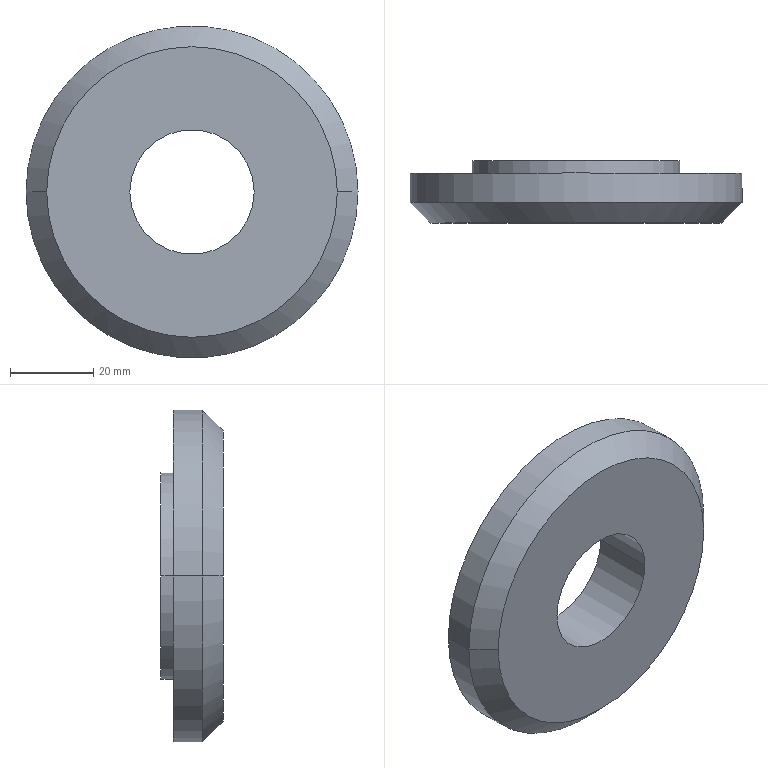Part | SolidWorks | features Revolution 1 | 1 solid | 14 faces | box 80 x 15 x 80 mm | volume 46941 mm3 | cylinder 8 | plane 4 | cone 2 | commonest cylinder face diameters 30 x2 50 x2 70 x2 80 x2
STEP:
#1=CARTESIAN_POINT('',(25.,532.,0.));
#2=VERTEX_POINT('',#1);
#3=CARTESIAN_POINT('',(-25.,532.,0.));
#4=VERTEX_POINT('',#3);
#5=CARTESIAN_POINT('',(0.,532.,0.));
#6=DIRECTION('',(0.,-1.,0.));
#7=DIRECTION('',(1.,0.,0.));
#8=AXIS2_PLACEMENT_3D('',#5,#6,#7);
#9=CIRCLE('',#8,25.);
#10=EDGE_CURVE('',#2,#4,#9,.T.);
#11=ORIENTED_EDGE('',*,*,#10,.T.);
#12=CARTESIAN_POINT('',(-25.,526.,0.));
#13=VERTEX_POINT('',#12);
#14=CARTESIAN_POINT('',(-25.,517.,0.));
#15=DIRECTION('',(0.,-1.,0.));
#16=VECTOR('',#15,1000.);
#17=LINE('',#14,#16);
#18=EDGE_CURVE('',#4,#13,#17,.T.);
#19=ORIENTED_EDGE('',*,*,#18,.T.);
#20=CARTESIAN_POINT('',(25.,526.,0.));
#21=VERTEX_POINT('',#20);
#22=CARTESIAN_POINT('',(0.,526.,0.));
#23=DIRECTION('',(0.,-1.,0.));
#24=DIRECTION('',(1.,0.,0.));
#25=AXIS2_PLACEMENT_3D('',#22,#23,#24);
#26=CIRCLE('',#25,25.);
#27=EDGE_CURVE('',#21,#13,#26,.T.);
#28=ORIENTED_EDGE('',*,*,#27,.F.);
#29=CARTESIAN_POINT('',(25.,517.,0.));
#30=DIRECTION('',(0.,-1.,0.));
#31=VECTOR('',#30,1000.);
#32=LINE('',#29,#31);
#33=EDGE_CURVE('',#2,#21,#32,.T.);
#34=ORIENTED_EDGE('',*,*,#33,.F.);
#35=EDGE_LOOP('',(#11,#19,#28,#34));
#36=FACE_OUTER_BOUND('',#35,.T.);
#37=CARTESIAN_POINT('',(0.,517.,0.));
#38=DIRECTION('',(0.,-1.,0.));
#39=DIRECTION('',(1.,0.,0.));
#40=AXIS2_PLACEMENT_3D('',#37,#38,#39);
#41=CYLINDRICAL_SURFACE('',#40,25.);
#42=ADVANCED_FACE('',(#36),#41,.T.);
#43=CARTESIAN_POINT('',(-35.,529.,0.));
#44=VERTEX_POINT('',#43);
#45=CARTESIAN_POINT('',(35.,529.,0.));
#46=VERTEX_POINT('',#45);
#47=CARTESIAN_POINT('',(0.,529.,0.));
#48=DIRECTION('',(0.,-1.,0.));
#49=DIRECTION('',(1.,0.,0.));
#50=AXIS2_PLACEMENT_3D('',#47,#48,#49);
#51=CIRCLE('',#50,35.);
#52=EDGE_CURVE('',#44,#46,#51,.T.);
#53=ORIENTED_EDGE('',*,*,#52,.F.);
#54=CARTESIAN_POINT('',(-35.,526.,0.));
#55=VERTEX_POINT('',#54);
#56=CARTESIAN_POINT('',(-35.,517.,0.));
#57=DIRECTION('',(0.,-1.,0.));
#58=VECTOR('',#57,1000.);
#59=LINE('',#56,#58);
#60=EDGE_CURVE('',#44,#55,#59,.T.);
#61=ORIENTED_EDGE('',*,*,#60,.T.);
#62=CARTESIAN_POINT('',(35.,526.,0.));
#63=VERTEX_POINT('',#62);
#64=CARTESIAN_POINT('',(0.,526.,0.));
#65=DIRECTION('',(0.,-1.,0.));
#66=DIRECTION('',(1.,0.,0.));
#67=AXIS2_PLACEMENT_3D('',#64,#65,#66);
#68=CIRCLE('',#67,35.);
#69=EDGE_CURVE('',#55,#63,#68,.T.);
#70=ORIENTED_EDGE('',*,*,#69,.T.);
#71=CARTESIAN_POINT('',(35.,517.,0.));
#72=DIRECTION('',(0.,-1.,0.));
#73=VECTOR('',#72,1000.);
#74=LINE('',#71,#73);
#75=EDGE_CURVE('',#46,#63,#74,.T.);
#76=ORIENTED_EDGE('',*,*,#75,.F.);
#77=EDGE_LOOP('',(#53,#61,#70,#76));
#78=FACE_OUTER_BOUND('',#77,.T.);
#79=CARTESIAN_POINT('',(0.,517.,0.));
#80=DIRECTION('',(0.,-1.,0.));
#81=DIRECTION('',(1.,0.,0.));
#82=AXIS2_PLACEMENT_3D('',#79,#80,#81);
#83=CYLINDRICAL_SURFACE('',#82,35.);
#84=ADVANCED_FACE('',(#78),#83,.F.);
#85=CARTESIAN_POINT('',(40.,529.,0.));
#86=VERTEX_POINT('',#85);
#87=CARTESIAN_POINT('',(-40.,529.,0.));
#88=VERTEX_POINT('',#87);
#89=CARTESIAN_POINT('',(0.,529.,0.));
#90=DIRECTION('',(0.,-1.,0.));
#91=DIRECTION('',(1.,0.,0.));
#92=AXIS2_PLACEMENT_3D('',#89,#90,#91);
#93=CIRCLE('',#92,40.);
#94=EDGE_CURVE('',#86,#88,#93,.T.);
#95=ORIENTED_EDGE('',*,*,#94,.T.);
#96=CARTESIAN_POINT('',(-40.,522.,0.));
#97=VERTEX_POINT('',#96);
#98=CARTESIAN_POINT('',(-40.,517.,0.));
#99=DIRECTION('',(0.,-1.,0.));
#100=VECTOR('',#99,1000.);
#101=LINE('',#98,#100);
#102=EDGE_CURVE('',#88,#97,#101,.T.);
#103=ORIENTED_EDGE('',*,*,#102,.T.);
#104=CARTESIAN_POINT('',(40.,522.,0.));
#105=VERTEX_POINT('',#104);
#106=CARTESIAN_POINT('',(0.,522.,0.));
#107=DIRECTION('',(0.,-1.,0.));
#108=DIRECTION('',(1.,0.,0.));
#109=AXIS2_PLACEMENT_3D('',#106,#107,#108);
#110=CIRCLE('',#109,40.);
#111=EDGE_CURVE('',#105,#97,#110,.T.);
#112=ORIENTED_EDGE('',*,*,#111,.F.);
#113=CARTESIAN_POINT('',(40.,517.,0.));
#114=DIRECTION('',(0.,-1.,0.));
#115=VECTOR('',#114,1000.);
#116=LINE('',#113,#115);
#117=EDGE_CURVE('',#86,#105,#116,.T.);
#118=ORIENTED_EDGE('',*,*,#117,.F.);
#119=EDGE_LOOP('',(#95,#103,#112,#118));
#120=FACE_OUTER_BOUND('',#119,.T.);
#121=CARTESIAN_POINT('',(0.,517.,0.));
#122=DIRECTION('',(0.,-1.,0.));
#123=DIRECTION('',(1.,0.,0.));
#124=AXIS2_PLACEMENT_3D('',#121,#122,#123);
#125=CYLINDRICAL_SURFACE('',#124,40.);
#126=ADVANCED_FACE('',(#120),#125,.T.);
#127=CARTESIAN_POINT('',(35.,517.,0.));
#128=VERTEX_POINT('',#127);
#129=CARTESIAN_POINT('',(-35.,517.,0.));
#130=VERTEX_POINT('',#129);
#131=CARTESIAN_POINT('',(0.,517.,0.));
#132=DIRECTION('',(0.,-1.,0.));
#133=DIRECTION('',(1.,0.,0.));
#134=AXIS2_PLACEMENT_3D('',#131,#132,#133);
#135=CIRCLE('',#134,35.);
#136=EDGE_CURVE('',#128,#130,#135,.T.);
#137=ORIENTED_EDGE('',*,*,#136,.F.);
#138=CARTESIAN_POINT('',(35.,517.,0.));
#139=DIRECTION('',(0.7071,0.7071,0.));
#140=VECTOR('',#139,1000.);
#141=LINE('',#138,#140);
#142=EDGE_CURVE('',#128,#105,#141,.T.);
#143=ORIENTED_EDGE('',*,*,#142,.T.);
#144=ORIENTED_EDGE('',*,*,#111,.T.);
#145=CARTESIAN_POINT('',(-35.,517.,0.));
#146=DIRECTION('',(-0.7071,0.7071,0.));
#147=VECTOR('',#146,1000.);
#148=LINE('',#145,#147);
#149=EDGE_CURVE('',#130,#97,#148,.T.);
#150=ORIENTED_EDGE('',*,*,#149,.F.);
#151=EDGE_LOOP('',(#137,#143,#144,#150));
#152=FACE_OUTER_BOUND('',#151,.T.);
#153=CARTESIAN_POINT('',(0.,517.,0.));
#154=DIRECTION('',(0.,1.,0.));
#155=DIRECTION('',(-1.,0.,0.));
#156=AXIS2_PLACEMENT_3D('',#153,#154,#155);
#157=CONICAL_SURFACE('',#156,35.,0.7854);
#158=ADVANCED_FACE('',(#152),#157,.T.);
#159=CARTESIAN_POINT('',(-15.,532.,0.));
#160=VERTEX_POINT('',#159);
#161=CARTESIAN_POINT('',(15.,532.,0.));
#162=VERTEX_POINT('',#161);
#163=CARTESIAN_POINT('',(0.,532.,0.));
#164=DIRECTION('',(0.,-1.,0.));
#165=DIRECTION('',(1.,0.,0.));
#166=AXIS2_PLACEMENT_3D('',#163,#164,#165);
#167=CIRCLE('',#166,15.);
#168=EDGE_CURVE('',#160,#162,#167,.T.);
#169=ORIENTED_EDGE('',*,*,#168,.F.);
#170=CARTESIAN_POINT('',(-15.,517.,0.));
#171=VERTEX_POINT('',#170);
#172=CARTESIAN_POINT('',(-15.,517.,0.));
#173=DIRECTION('',(0.,-1.,0.));
#174=VECTOR('',#173,1000.);
#175=LINE('',#172,#174);
#176=EDGE_CURVE('',#160,#171,#175,.T.);
#177=ORIENTED_EDGE('',*,*,#176,.T.);
#178=CARTESIAN_POINT('',(15.,517.,0.));
#179=VERTEX_POINT('',#178);
#180=CARTESIAN_POINT('',(0.,517.,0.));
#181=DIRECTION('',(0.,-1.,0.));
#182=DIRECTION('',(1.,0.,0.));
#183=AXIS2_PLACEMENT_3D('',#180,#181,#182);
#184=CIRCLE('',#183,15.);
#185=EDGE_CURVE('',#171,#179,#184,.T.);
#186=ORIENTED_EDGE('',*,*,#185,.T.);
#187=CARTESIAN_POINT('',(15.,517.,0.));
#188=DIRECTION('',(0.,-1.,0.));
#189=VECTOR('',#188,1000.);
#190=LINE('',#187,#189);
#191=EDGE_CURVE('',#162,#179,#190,.T.);
#192=ORIENTED_EDGE('',*,*,#191,.F.);
#193=EDGE_LOOP('',(#169,#177,#186,#192));
#194=FACE_OUTER_BOUND('',#193,.T.);
#195=CARTESIAN_POINT('',(0.,517.,0.));
#196=DIRECTION('',(0.,-1.,0.));
#197=DIRECTION('',(1.,0.,0.));
#198=AXIS2_PLACEMENT_3D('',#195,#196,#197);
#199=CYLINDRICAL_SURFACE('',#198,15.);
#200=ADVANCED_FACE('',(#194),#199,.F.);
#201=ORIENTED_EDGE('',*,*,#176,.F.);
#202=CARTESIAN_POINT('',(0.,532.,0.));
#203=DIRECTION('',(0.,-1.,0.));
#204=DIRECTION('',(1.,0.,0.));
#205=AXIS2_PLACEMENT_3D('',#202,#203,#204);
#206=CIRCLE('',#205,15.);
#207=EDGE_CURVE('',#162,#160,#206,.T.);
#208=ORIENTED_EDGE('',*,*,#207,.F.);
#209=ORIENTED_EDGE('',*,*,#191,.T.);
#210=CARTESIAN_POINT('',(0.,517.,0.));
#211=DIRECTION('',(0.,-1.,0.));
#212=DIRECTION('',(1.,0.,0.));
#213=AXIS2_PLACEMENT_3D('',#210,#211,#212);
#214=CIRCLE('',#213,15.);
#215=EDGE_CURVE('',#179,#171,#214,.T.);
#216=ORIENTED_EDGE('',*,*,#215,.T.);
#217=EDGE_LOOP('',(#201,#208,#209,#216));
#218=FACE_OUTER_BOUND('',#217,.T.);
#219=CARTESIAN_POINT('',(0.,517.,0.));
#220=DIRECTION('',(0.,-1.,0.));
#221=DIRECTION('',(1.,0.,0.));
#222=AXIS2_PLACEMENT_3D('',#219,#220,#221);
#223=CYLINDRICAL_SURFACE('',#222,15.);
#224=ADVANCED_FACE('',(#218),#223,.F.);
#225=CARTESIAN_POINT('',(0.,517.,0.));
#226=DIRECTION('',(0.,-1.,0.));
#227=DIRECTION('',(1.,0.,0.));
#228=AXIS2_PLACEMENT_3D('',#225,#226,#227);
#229=CIRCLE('',#228,35.);
#230=EDGE_CURVE('',#130,#128,#229,.T.);
#231=ORIENTED_EDGE('',*,*,#230,.T.);
#232=ORIENTED_EDGE('',*,*,#136,.T.);
#233=EDGE_LOOP('',(#231,#232));
#234=FACE_OUTER_BOUND('',#233,.T.);
#235=ORIENTED_EDGE('',*,*,#215,.F.);
#236=ORIENTED_EDGE('',*,*,#185,.F.);
#237=EDGE_LOOP('',(#235,#236));
#238=FACE_BOUND('',#237,.T.);
#239=CARTESIAN_POINT('',(15.,517.,0.));
#240=DIRECTION('',(0.,-1.,0.));
#241=DIRECTION('',(1.,0.,0.));
#242=AXIS2_PLACEMENT_3D('',#239,#240,#241);
#243=PLANE('',#242);
#244=ADVANCED_FACE('',(#234,#238),#243,.T.);
#245=ORIENTED_EDGE('',*,*,#142,.F.);
#246=ORIENTED_EDGE('',*,*,#230,.F.);
#247=ORIENTED_EDGE('',*,*,#149,.T.);
#248=CARTESIAN_POINT('',(0.,522.,0.));
#249=DIRECTION('',(0.,-1.,0.));
#250=DIRECTION('',(1.,0.,0.));
#251=AXIS2_PLACEMENT_3D('',#248,#249,#250);
#252=CIRCLE('',#251,40.);
#253=EDGE_CURVE('',#97,#105,#252,.T.);
#254=ORIENTED_EDGE('',*,*,#253,.T.);
#255=EDGE_LOOP('',(#245,#246,#247,#254));
#256=FACE_OUTER_BOUND('',#255,.T.);
#257=CARTESIAN_POINT('',(0.,517.,0.));
#258=DIRECTION('',(0.,1.,0.));
#259=DIRECTION('',(-1.,0.,0.));
#260=AXIS2_PLACEMENT_3D('',#257,#258,#259);
#261=CONICAL_SURFACE('',#260,35.,0.7854);
#262=ADVANCED_FACE('',(#256),#261,.T.);
#263=ORIENTED_EDGE('',*,*,#102,.F.);
#264=CARTESIAN_POINT('',(0.,529.,0.));
#265=DIRECTION('',(0.,-1.,0.));
#266=DIRECTION('',(1.,0.,0.));
#267=AXIS2_PLACEMENT_3D('',#264,#265,#266);
#268=CIRCLE('',#267,40.);
#269=EDGE_CURVE('',#88,#86,#268,.T.);
#270=ORIENTED_EDGE('',*,*,#269,.T.);
#271=ORIENTED_EDGE('',*,*,#117,.T.);
#272=ORIENTED_EDGE('',*,*,#253,.F.);
#273=EDGE_LOOP('',(#263,#270,#271,#272));
#274=FACE_OUTER_BOUND('',#273,.T.);
#275=CARTESIAN_POINT('',(0.,517.,0.));
#276=DIRECTION('',(0.,-1.,0.));
#277=DIRECTION('',(1.,0.,0.));
#278=AXIS2_PLACEMENT_3D('',#275,#276,#277);
#279=CYLINDRICAL_SURFACE('',#278,40.);
#280=ADVANCED_FACE('',(#274),#279,.T.);
#281=CARTESIAN_POINT('',(0.,529.,0.));
#282=DIRECTION('',(0.,-1.,0.));
#283=DIRECTION('',(1.,0.,0.));
#284=AXIS2_PLACEMENT_3D('',#281,#282,#283);
#285=CIRCLE('',#284,35.);
#286=EDGE_CURVE('',#46,#44,#285,.T.);
#287=ORIENTED_EDGE('',*,*,#286,.T.);
#288=ORIENTED_EDGE('',*,*,#52,.T.);
#289=EDGE_LOOP('',(#287,#288));
#290=FACE_BOUND('',#289,.T.);
#291=ORIENTED_EDGE('',*,*,#94,.F.);
#292=ORIENTED_EDGE('',*,*,#269,.F.);
#293=EDGE_LOOP('',(#291,#292));
#294=FACE_OUTER_BOUND('',#293,.T.);
#295=CARTESIAN_POINT('',(40.,529.,0.));
#296=DIRECTION('',(0.,1.,0.));
#297=DIRECTION('',(-1.,0.,0.));
#298=AXIS2_PLACEMENT_3D('',#295,#296,#297);
#299=PLANE('',#298);
#300=ADVANCED_FACE('',(#290,#294),#299,.T.);
#301=ORIENTED_EDGE('',*,*,#60,.F.);
#302=ORIENTED_EDGE('',*,*,#286,.F.);
#303=ORIENTED_EDGE('',*,*,#75,.T.);
#304=CARTESIAN_POINT('',(0.,526.,0.));
#305=DIRECTION('',(0.,-1.,0.));
#306=DIRECTION('',(1.,0.,0.));
#307=AXIS2_PLACEMENT_3D('',#304,#305,#306);
#308=CIRCLE('',#307,35.);
#309=EDGE_CURVE('',#63,#55,#308,.T.);
#310=ORIENTED_EDGE('',*,*,#309,.T.);
#311=EDGE_LOOP('',(#301,#302,#303,#310));
#312=FACE_OUTER_BOUND('',#311,.T.);
#313=CARTESIAN_POINT('',(0.,517.,0.));
#314=DIRECTION('',(0.,-1.,0.));
#315=DIRECTION('',(1.,0.,0.));
#316=AXIS2_PLACEMENT_3D('',#313,#314,#315);
#317=CYLINDRICAL_SURFACE('',#316,35.);
#318=ADVANCED_FACE('',(#312),#317,.F.);
#319=ORIENTED_EDGE('',*,*,#27,.T.);
#320=CARTESIAN_POINT('',(0.,526.,0.));
#321=DIRECTION('',(0.,-1.,0.));
#322=DIRECTION('',(1.,0.,0.));
#323=AXIS2_PLACEMENT_3D('',#320,#321,#322);
#324=CIRCLE('',#323,25.);
#325=EDGE_CURVE('',#13,#21,#324,.T.);
#326=ORIENTED_EDGE('',*,*,#325,.T.);
#327=EDGE_LOOP('',(#319,#326));
#328=FACE_BOUND('',#327,.T.);
#329=ORIENTED_EDGE('',*,*,#309,.F.);
#330=ORIENTED_EDGE('',*,*,#69,.F.);
#331=EDGE_LOOP('',(#329,#330));
#332=FACE_OUTER_BOUND('',#331,.T.);
#333=CARTESIAN_POINT('',(35.,526.,0.));
#334=DIRECTION('',(0.,1.,0.));
#335=DIRECTION('',(-1.,0.,0.));
#336=AXIS2_PLACEMENT_3D('',#333,#334,#335);
#337=PLANE('',#336);
#338=ADVANCED_FACE('',(#328,#332),#337,.T.);
#339=ORIENTED_EDGE('',*,*,#18,.F.);
#340=CARTESIAN_POINT('',(0.,532.,0.));
#341=DIRECTION('',(0.,-1.,0.));
#342=DIRECTION('',(1.,0.,0.));
#343=AXIS2_PLACEMENT_3D('',#340,#341,#342);
#344=CIRCLE('',#343,25.);
#345=EDGE_CURVE('',#4,#2,#344,.T.);
#346=ORIENTED_EDGE('',*,*,#345,.T.);
#347=ORIENTED_EDGE('',*,*,#33,.T.);
#348=ORIENTED_EDGE('',*,*,#325,.F.);
#349=EDGE_LOOP('',(#339,#346,#347,#348));
#350=FACE_OUTER_BOUND('',#349,.T.);
#351=CARTESIAN_POINT('',(0.,517.,0.));
#352=DIRECTION('',(0.,-1.,0.));
#353=DIRECTION('',(1.,0.,0.));
#354=AXIS2_PLACEMENT_3D('',#351,#352,#353);
#355=CYLINDRICAL_SURFACE('',#354,25.);
#356=ADVANCED_FACE('',(#350),#355,.T.);
#357=ORIENTED_EDGE('',*,*,#207,.T.);
#358=ORIENTED_EDGE('',*,*,#168,.T.);
#359=EDGE_LOOP('',(#357,#358));
#360=FACE_BOUND('',#359,.T.);
#361=ORIENTED_EDGE('',*,*,#10,.F.);
#362=ORIENTED_EDGE('',*,*,#345,.F.);
#363=EDGE_LOOP('',(#361,#362));
#364=FACE_OUTER_BOUND('',#363,.T.);
#365=CARTESIAN_POINT('',(25.,532.,0.));
#366=DIRECTION('',(0.,1.,0.));
#367=DIRECTION('',(-1.,0.,0.));
#368=AXIS2_PLACEMENT_3D('',#365,#366,#367);
#369=PLANE('',#368);
#370=ADVANCED_FACE('',(#360,#364),#369,.T.);
#371=CLOSED_SHELL('',(#42,#84,#126,#158,#200,#224,#244,#262,#280,#300,#318,#338,#356,#370));
#372=MANIFOLD_SOLID_BREP('',#371);
#373=CARTESIAN_POINT('',(0.,0.,0.));
#374=DIRECTION('',(0.,0.,1.));
#375=DIRECTION('',(1.,0.,0.));
#376=AXIS2_PLACEMENT_3D('',#373,#374,#375);
#377=(LENGTH_UNIT()NAMED_UNIT(*)SI_UNIT(.MILLI.,.METRE.));
#378=UNCERTAINTY_MEASURE_WITH_UNIT(LENGTH_MEASURE(0.00001),#377,'','');
#379=(NAMED_UNIT(*)PLANE_ANGLE_UNIT()SI_UNIT($,.RADIAN.));
#380=(NAMED_UNIT(*)SI_UNIT($,.STERADIAN.)SOLID_ANGLE_UNIT());
#381=(GEOMETRIC_REPRESENTATION_CONTEXT(3)GLOBAL_UNCERTAINTY_ASSIGNED_CONTEXT((#378))GLOBAL_UNIT_ASSIGNED_CONTEXT((#377,#379,#380))REPRESENTATION_CONTEXT('',''));
#382=ADVANCED_BREP_SHAPE_REPRESENTATION('',(#372,#376),#381);